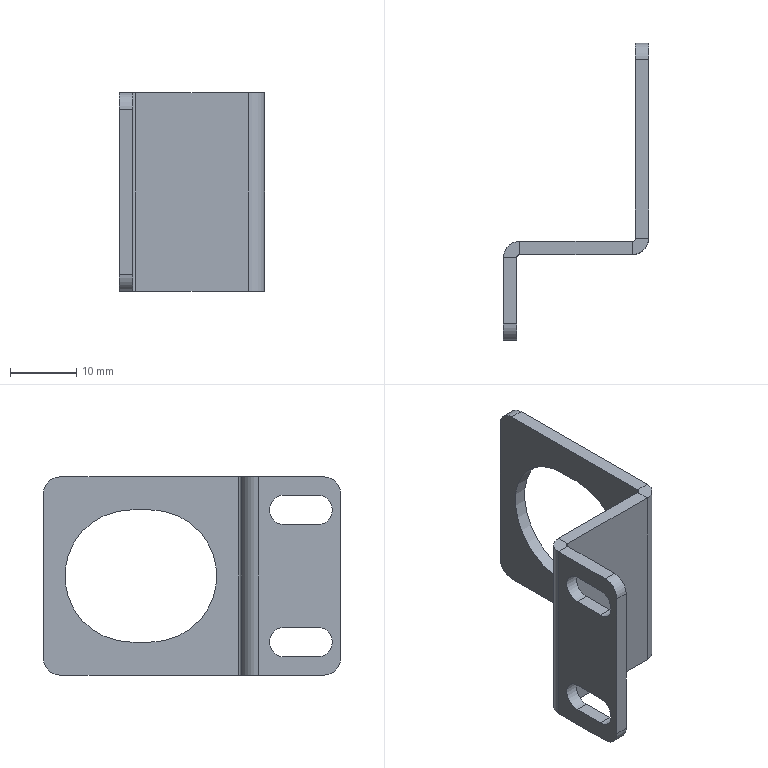Part | STEP file | KF-2212-070-008 | 1 solid | 38 faces | box 22 x 45 x 30 mm | volume 2910 mm3 | plane 24 | cylinder 14 | commonest cylinder face diameters 5 x6 4.5 x4 1 x2 20 x2
STEP:
#1=CARTESIAN_POINT('',(2.5,0.,30.));
#2=VERTEX_POINT('',#1);
#3=CARTESIAN_POINT('',(2.5,-2.,30.));
#4=VERTEX_POINT('',#3);
#5=CARTESIAN_POINT('',(2.5,0.,30.));
#6=DIRECTION('',(0.,-1.,0.));
#7=VECTOR('',#6,1000.);
#8=LINE('',#5,#7);
#9=EDGE_CURVE('',#2,#4,#8,.T.);
#10=ORIENTED_EDGE('',*,*,#9,.F.);
#11=CARTESIAN_POINT('',(0.,-2.5,30.));
#12=VERTEX_POINT('',#11);
#13=CARTESIAN_POINT('',(2.5,-2.5,30.));
#14=DIRECTION('',(0.,0.,-1.));
#15=DIRECTION('',(1.,0.,0.));
#16=AXIS2_PLACEMENT_3D('',#13,#14,#15);
#17=CIRCLE('',#16,2.5);
#18=EDGE_CURVE('',#12,#2,#17,.T.);
#19=ORIENTED_EDGE('',*,*,#18,.F.);
#20=CARTESIAN_POINT('',(2.,-2.5,30.));
#21=VERTEX_POINT('',#20);
#22=CARTESIAN_POINT('',(2.,-2.5,30.));
#23=DIRECTION('',(-1.,0.,0.));
#24=VECTOR('',#23,1000.);
#25=LINE('',#22,#24);
#26=EDGE_CURVE('',#21,#12,#25,.T.);
#27=ORIENTED_EDGE('',*,*,#26,.F.);
#28=CARTESIAN_POINT('',(2.5,-2.5,30.));
#29=DIRECTION('',(0.,0.,-1.));
#30=DIRECTION('',(1.,0.,0.));
#31=AXIS2_PLACEMENT_3D('',#28,#29,#30);
#32=CIRCLE('',#31,0.5);
#33=EDGE_CURVE('',#21,#4,#32,.T.);
#34=ORIENTED_EDGE('',*,*,#33,.T.);
#35=EDGE_LOOP('',(#10,#19,#27,#34));
#36=FACE_OUTER_BOUND('',#35,.T.);
#37=CARTESIAN_POINT('',(2.5,0.,30.));
#38=DIRECTION('',(0.,0.,1.));
#39=DIRECTION('',(1.,0.,0.));
#40=AXIS2_PLACEMENT_3D('',#37,#38,#39);
#41=PLANE('',#40);
#42=ADVANCED_FACE('',(#36),#41,.T.);
#43=CARTESIAN_POINT('',(19.5,0.,30.));
#44=VERTEX_POINT('',#43);
#45=CARTESIAN_POINT('',(0.,0.,30.));
#46=DIRECTION('',(1.,0.,0.));
#47=VECTOR('',#46,1000.);
#48=LINE('',#45,#47);
#49=EDGE_CURVE('',#2,#44,#48,.T.);
#50=ORIENTED_EDGE('',*,*,#49,.F.);
#51=ORIENTED_EDGE('',*,*,#9,.T.);
#52=CARTESIAN_POINT('',(19.5,-2.,30.));
#53=VERTEX_POINT('',#52);
#54=CARTESIAN_POINT('',(0.,-2.,30.));
#55=DIRECTION('',(1.,0.,0.));
#56=VECTOR('',#55,1000.);
#57=LINE('',#54,#56);
#58=EDGE_CURVE('',#4,#53,#57,.T.);
#59=ORIENTED_EDGE('',*,*,#58,.T.);
#60=CARTESIAN_POINT('',(19.5,-2.,30.));
#61=DIRECTION('',(0.,1.,0.));
#62=VECTOR('',#61,1000.);
#63=LINE('',#60,#62);
#64=EDGE_CURVE('',#53,#44,#63,.T.);
#65=ORIENTED_EDGE('',*,*,#64,.T.);
#66=EDGE_LOOP('',(#50,#51,#59,#65));
#67=FACE_OUTER_BOUND('',#66,.T.);
#68=CARTESIAN_POINT('',(2.,-2.5,30.));
#69=DIRECTION('',(0.,0.,1.));
#70=DIRECTION('',(1.,0.,0.));
#71=AXIS2_PLACEMENT_3D('',#68,#69,#70);
#72=PLANE('',#71);
#73=ADVANCED_FACE('',(#67),#72,.T.);
#74=CARTESIAN_POINT('',(0.,-2.5,0.));
#75=VERTEX_POINT('',#74);
#76=CARTESIAN_POINT('',(2.,-2.5,0.));
#77=VERTEX_POINT('',#76);
#78=CARTESIAN_POINT('',(0.,-2.5,0.));
#79=DIRECTION('',(1.,0.,0.));
#80=VECTOR('',#79,1000.);
#81=LINE('',#78,#80);
#82=EDGE_CURVE('',#75,#77,#81,.T.);
#83=ORIENTED_EDGE('',*,*,#82,.F.);
#84=CARTESIAN_POINT('',(2.5,0.,0.));
#85=VERTEX_POINT('',#84);
#86=CARTESIAN_POINT('',(2.5,-2.5,0.));
#87=DIRECTION('',(0.,0.,-1.));
#88=DIRECTION('',(1.,0.,0.));
#89=AXIS2_PLACEMENT_3D('',#86,#87,#88);
#90=CIRCLE('',#89,2.5);
#91=EDGE_CURVE('',#75,#85,#90,.T.);
#92=ORIENTED_EDGE('',*,*,#91,.T.);
#93=CARTESIAN_POINT('',(2.5,-2.,0.));
#94=VERTEX_POINT('',#93);
#95=CARTESIAN_POINT('',(2.5,-2.,0.));
#96=DIRECTION('',(0.,1.,0.));
#97=VECTOR('',#96,1000.);
#98=LINE('',#95,#97);
#99=EDGE_CURVE('',#94,#85,#98,.T.);
#100=ORIENTED_EDGE('',*,*,#99,.F.);
#101=CARTESIAN_POINT('',(2.5,-2.5,0.));
#102=DIRECTION('',(0.,0.,-1.));
#103=DIRECTION('',(1.,0.,0.));
#104=AXIS2_PLACEMENT_3D('',#101,#102,#103);
#105=CIRCLE('',#104,0.5);
#106=EDGE_CURVE('',#77,#94,#105,.T.);
#107=ORIENTED_EDGE('',*,*,#106,.F.);
#108=EDGE_LOOP('',(#83,#92,#100,#107));
#109=FACE_OUTER_BOUND('',#108,.T.);
#110=CARTESIAN_POINT('',(0.,-2.5,0.));
#111=DIRECTION('',(0.,0.,-1.));
#112=DIRECTION('',(-1.,0.,0.));
#113=AXIS2_PLACEMENT_3D('',#110,#111,#112);
#114=PLANE('',#113);
#115=ADVANCED_FACE('',(#109),#114,.T.);
#116=CARTESIAN_POINT('',(2.,-12.5,0.));
#117=VERTEX_POINT('',#116);
#118=CARTESIAN_POINT('',(2.,-15.,0.));
#119=DIRECTION('',(0.,1.,0.));
#120=VECTOR('',#119,1000.);
#121=LINE('',#118,#120);
#122=EDGE_CURVE('',#117,#77,#121,.T.);
#123=ORIENTED_EDGE('',*,*,#122,.F.);
#124=CARTESIAN_POINT('',(0.,-12.5,0.));
#125=VERTEX_POINT('',#124);
#126=CARTESIAN_POINT('',(2.5,-12.5,0.));
#127=DIRECTION('',(-1.,0.,0.));
#128=VECTOR('',#127,1000.);
#129=LINE('',#126,#128);
#130=EDGE_CURVE('',#117,#125,#129,.T.);
#131=ORIENTED_EDGE('',*,*,#130,.T.);
#132=CARTESIAN_POINT('',(0.,-15.,0.));
#133=DIRECTION('',(0.,1.,0.));
#134=VECTOR('',#133,1000.);
#135=LINE('',#132,#134);
#136=EDGE_CURVE('',#125,#75,#135,.T.);
#137=ORIENTED_EDGE('',*,*,#136,.T.);
#138=ORIENTED_EDGE('',*,*,#82,.T.);
#139=EDGE_LOOP('',(#123,#131,#137,#138));
#140=FACE_OUTER_BOUND('',#139,.T.);
#141=CARTESIAN_POINT('',(2.5,-2.,0.));
#142=DIRECTION('',(0.,0.,-1.));
#143=DIRECTION('',(-1.,0.,0.));
#144=AXIS2_PLACEMENT_3D('',#141,#142,#143);
#145=PLANE('',#144);
#146=ADVANCED_FACE('',(#140),#145,.T.);
#147=CARTESIAN_POINT('',(20.,0.5,30.));
#148=VERTEX_POINT('',#147);
#149=CARTESIAN_POINT('',(22.,0.5,30.));
#150=VERTEX_POINT('',#149);
#151=CARTESIAN_POINT('',(20.,0.5,30.));
#152=DIRECTION('',(1.,0.,0.));
#153=VECTOR('',#152,1000.);
#154=LINE('',#151,#153);
#155=EDGE_CURVE('',#148,#150,#154,.T.);
#156=ORIENTED_EDGE('',*,*,#155,.F.);
#157=CARTESIAN_POINT('',(19.5,0.5,30.));
#158=DIRECTION('',(0.,0.,1.));
#159=DIRECTION('',(-1.,0.,0.));
#160=AXIS2_PLACEMENT_3D('',#157,#158,#159);
#161=CIRCLE('',#160,0.5);
#162=EDGE_CURVE('',#44,#148,#161,.T.);
#163=ORIENTED_EDGE('',*,*,#162,.F.);
#164=ORIENTED_EDGE('',*,*,#64,.F.);
#165=CARTESIAN_POINT('',(19.5,0.5,30.));
#166=DIRECTION('',(0.,0.,1.));
#167=DIRECTION('',(1.,0.,0.));
#168=AXIS2_PLACEMENT_3D('',#165,#166,#167);
#169=CIRCLE('',#168,2.5);
#170=EDGE_CURVE('',#53,#150,#169,.T.);
#171=ORIENTED_EDGE('',*,*,#170,.T.);
#172=EDGE_LOOP('',(#156,#163,#164,#171));
#173=FACE_OUTER_BOUND('',#172,.T.);
#174=CARTESIAN_POINT('',(20.,0.5,30.));
#175=DIRECTION('',(0.,0.,1.));
#176=DIRECTION('',(1.,0.,0.));
#177=AXIS2_PLACEMENT_3D('',#174,#175,#176);
#178=PLANE('',#177);
#179=ADVANCED_FACE('',(#173),#178,.T.);
#180=CARTESIAN_POINT('',(22.,27.5,30.));
#181=VERTEX_POINT('',#180);
#182=CARTESIAN_POINT('',(22.,0.,30.));
#183=DIRECTION('',(0.,1.,0.));
#184=VECTOR('',#183,1000.);
#185=LINE('',#182,#184);
#186=EDGE_CURVE('',#150,#181,#185,.T.);
#187=ORIENTED_EDGE('',*,*,#186,.T.);
#188=CARTESIAN_POINT('',(20.,27.5,30.));
#189=VERTEX_POINT('',#188);
#190=CARTESIAN_POINT('',(19.5,27.5,30.));
#191=DIRECTION('',(-1.,0.,0.));
#192=VECTOR('',#191,1000.);
#193=LINE('',#190,#192);
#194=EDGE_CURVE('',#181,#189,#193,.T.);
#195=ORIENTED_EDGE('',*,*,#194,.T.);
#196=CARTESIAN_POINT('',(20.,0.,30.));
#197=DIRECTION('',(0.,1.,0.));
#198=VECTOR('',#197,1000.);
#199=LINE('',#196,#198);
#200=EDGE_CURVE('',#148,#189,#199,.T.);
#201=ORIENTED_EDGE('',*,*,#200,.F.);
#202=ORIENTED_EDGE('',*,*,#155,.T.);
#203=EDGE_LOOP('',(#187,#195,#201,#202));
#204=FACE_OUTER_BOUND('',#203,.T.);
#205=CARTESIAN_POINT('',(19.5,-2.,30.));
#206=DIRECTION('',(0.,0.,1.));
#207=DIRECTION('',(1.,0.,0.));
#208=AXIS2_PLACEMENT_3D('',#205,#206,#207);
#209=PLANE('',#208);
#210=ADVANCED_FACE('',(#204),#209,.T.);
#211=CARTESIAN_POINT('',(19.5,0.,0.));
#212=VERTEX_POINT('',#211);
#213=CARTESIAN_POINT('',(19.5,-2.,0.));
#214=VERTEX_POINT('',#213);
#215=CARTESIAN_POINT('',(19.5,0.,0.));
#216=DIRECTION('',(0.,-1.,0.));
#217=VECTOR('',#216,1000.);
#218=LINE('',#215,#217);
#219=EDGE_CURVE('',#212,#214,#218,.T.);
#220=ORIENTED_EDGE('',*,*,#219,.F.);
#221=CARTESIAN_POINT('',(20.,0.5,0.));
#222=VERTEX_POINT('',#221);
#223=CARTESIAN_POINT('',(19.5,0.5,0.));
#224=DIRECTION('',(0.,0.,1.));
#225=DIRECTION('',(-1.,0.,0.));
#226=AXIS2_PLACEMENT_3D('',#223,#224,#225);
#227=CIRCLE('',#226,0.5);
#228=EDGE_CURVE('',#212,#222,#227,.T.);
#229=ORIENTED_EDGE('',*,*,#228,.T.);
#230=CARTESIAN_POINT('',(22.,0.5,0.));
#231=VERTEX_POINT('',#230);
#232=CARTESIAN_POINT('',(22.,0.5,0.));
#233=DIRECTION('',(-1.,0.,0.));
#234=VECTOR('',#233,1000.);
#235=LINE('',#232,#234);
#236=EDGE_CURVE('',#231,#222,#235,.T.);
#237=ORIENTED_EDGE('',*,*,#236,.F.);
#238=CARTESIAN_POINT('',(19.5,0.5,0.));
#239=DIRECTION('',(0.,0.,1.));
#240=DIRECTION('',(1.,0.,0.));
#241=AXIS2_PLACEMENT_3D('',#238,#239,#240);
#242=CIRCLE('',#241,2.5);
#243=EDGE_CURVE('',#214,#231,#242,.T.);
#244=ORIENTED_EDGE('',*,*,#243,.F.);
#245=EDGE_LOOP('',(#220,#229,#237,#244));
#246=FACE_OUTER_BOUND('',#245,.T.);
#247=CARTESIAN_POINT('',(19.5,0.,0.));
#248=DIRECTION('',(0.,0.,-1.));
#249=DIRECTION('',(-1.,0.,0.));
#250=AXIS2_PLACEMENT_3D('',#247,#248,#249);
#251=PLANE('',#250);
#252=ADVANCED_FACE('',(#246),#251,.T.);
#253=CARTESIAN_POINT('',(0.,0.,0.));
#254=DIRECTION('',(1.,0.,0.));
#255=VECTOR('',#254,1000.);
#256=LINE('',#253,#255);
#257=EDGE_CURVE('',#85,#212,#256,.T.);
#258=ORIENTED_EDGE('',*,*,#257,.T.);
#259=ORIENTED_EDGE('',*,*,#219,.T.);
#260=CARTESIAN_POINT('',(0.,-2.,0.));
#261=DIRECTION('',(1.,0.,0.));
#262=VECTOR('',#261,1000.);
#263=LINE('',#260,#262);
#264=EDGE_CURVE('',#94,#214,#263,.T.);
#265=ORIENTED_EDGE('',*,*,#264,.F.);
#266=ORIENTED_EDGE('',*,*,#99,.T.);
#267=EDGE_LOOP('',(#258,#259,#265,#266));
#268=FACE_OUTER_BOUND('',#267,.T.);
#269=CARTESIAN_POINT('',(22.,0.5,0.));
#270=DIRECTION('',(0.,0.,-1.));
#271=DIRECTION('',(-1.,0.,0.));
#272=AXIS2_PLACEMENT_3D('',#269,#270,#271);
#273=PLANE('',#272);
#274=ADVANCED_FACE('',(#268),#273,.T.);
#275=CARTESIAN_POINT('',(22.,16.75,25.));
#276=VERTEX_POINT('',#275);
#277=CARTESIAN_POINT('',(22.,13.75,25.));
#278=VERTEX_POINT('',#277);
#279=CARTESIAN_POINT('',(22.,16.75,25.));
#280=DIRECTION('',(0.,-1.,0.));
#281=VECTOR('',#280,1000.);
#282=LINE('',#279,#281);
#283=EDGE_CURVE('',#276,#278,#282,.T.);
#284=ORIENTED_EDGE('',*,*,#283,.F.);
#285=CARTESIAN_POINT('',(22.,16.75,5.));
#286=VERTEX_POINT('',#285);
#287=CARTESIAN_POINT('',(22.,16.75,15.));
#288=DIRECTION('',(1.,0.,0.));
#289=DIRECTION('',(0.,0.,-1.));
#290=AXIS2_PLACEMENT_3D('',#287,#288,#289);
#291=CIRCLE('',#290,10.);
#292=EDGE_CURVE('',#286,#276,#291,.T.);
#293=ORIENTED_EDGE('',*,*,#292,.F.);
#294=CARTESIAN_POINT('',(22.,13.75,5.));
#295=VERTEX_POINT('',#294);
#296=CARTESIAN_POINT('',(22.,16.75,5.));
#297=DIRECTION('',(0.,1.,0.));
#298=VECTOR('',#297,1000.);
#299=LINE('',#296,#298);
#300=EDGE_CURVE('',#295,#286,#299,.T.);
#301=ORIENTED_EDGE('',*,*,#300,.F.);
#302=CARTESIAN_POINT('',(22.,13.75,15.));
#303=DIRECTION('',(1.,0.,0.));
#304=DIRECTION('',(0.,0.,-1.));
#305=AXIS2_PLACEMENT_3D('',#302,#303,#304);
#306=CIRCLE('',#305,10.);
#307=EDGE_CURVE('',#278,#295,#306,.T.);
#308=ORIENTED_EDGE('',*,*,#307,.F.);
#309=EDGE_LOOP('',(#284,#293,#301,#308));
#310=FACE_BOUND('',#309,.T.);
#311=CARTESIAN_POINT('',(22.,27.5,0.));
#312=VERTEX_POINT('',#311);
#313=CARTESIAN_POINT('',(22.,0.,0.));
#314=DIRECTION('',(0.,1.,0.));
#315=VECTOR('',#314,1000.);
#316=LINE('',#313,#315);
#317=EDGE_CURVE('',#231,#312,#316,.T.);
#318=ORIENTED_EDGE('',*,*,#317,.T.);
#319=CARTESIAN_POINT('',(22.,30.,2.5));
#320=VERTEX_POINT('',#319);
#321=CARTESIAN_POINT('',(22.,27.5,2.5));
#322=DIRECTION('',(1.,0.,0.));
#323=DIRECTION('',(0.,0.,1.));
#324=AXIS2_PLACEMENT_3D('',#321,#322,#323);
#325=CIRCLE('',#324,2.5);
#326=EDGE_CURVE('',#312,#320,#325,.T.);
#327=ORIENTED_EDGE('',*,*,#326,.T.);
#328=CARTESIAN_POINT('',(22.,30.,27.5));
#329=VERTEX_POINT('',#328);
#330=CARTESIAN_POINT('',(22.,30.,30.));
#331=DIRECTION('',(0.,0.,-1.));
#332=VECTOR('',#331,1000.);
#333=LINE('',#330,#332);
#334=EDGE_CURVE('',#329,#320,#333,.T.);
#335=ORIENTED_EDGE('',*,*,#334,.F.);
#336=CARTESIAN_POINT('',(22.,27.5,27.5));
#337=DIRECTION('',(1.,0.,0.));
#338=DIRECTION('',(0.,0.,1.));
#339=AXIS2_PLACEMENT_3D('',#336,#337,#338);
#340=CIRCLE('',#339,2.5);
#341=EDGE_CURVE('',#329,#181,#340,.T.);
#342=ORIENTED_EDGE('',*,*,#341,.T.);
#343=ORIENTED_EDGE('',*,*,#186,.F.);
#344=CARTESIAN_POINT('',(22.,0.5,30.));
#345=DIRECTION('',(0.,0.,-1.));
#346=VECTOR('',#345,1000.);
#347=LINE('',#344,#346);
#348=EDGE_CURVE('',#150,#231,#347,.T.);
#349=ORIENTED_EDGE('',*,*,#348,.T.);
#350=EDGE_LOOP('',(#318,#327,#335,#342,#343,#349));
#351=FACE_OUTER_BOUND('',#350,.T.);
#352=CARTESIAN_POINT('',(22.,0.,30.));
#353=DIRECTION('',(-1.,0.,0.));
#354=DIRECTION('',(0.,0.,1.));
#355=AXIS2_PLACEMENT_3D('',#352,#353,#354);
#356=PLANE('',#355);
#357=ADVANCED_FACE('',(#310,#351),#356,.F.);
#358=ORIENTED_EDGE('',*,*,#334,.T.);
#359=CARTESIAN_POINT('',(20.,30.,2.5));
#360=VERTEX_POINT('',#359);
#361=CARTESIAN_POINT('',(20.,30.,2.5));
#362=DIRECTION('',(-1.,0.,0.));
#363=VECTOR('',#362,1000.);
#364=LINE('',#361,#363);
#365=EDGE_CURVE('',#320,#360,#364,.T.);
#366=ORIENTED_EDGE('',*,*,#365,.T.);
#367=CARTESIAN_POINT('',(20.,30.,27.5));
#368=VERTEX_POINT('',#367);
#369=CARTESIAN_POINT('',(20.,30.,30.));
#370=DIRECTION('',(0.,0.,-1.));
#371=VECTOR('',#370,1000.);
#372=LINE('',#369,#371);
#373=EDGE_CURVE('',#368,#360,#372,.T.);
#374=ORIENTED_EDGE('',*,*,#373,.F.);
#375=CARTESIAN_POINT('',(20.,30.,27.5));
#376=DIRECTION('',(1.,0.,0.));
#377=VECTOR('',#376,1000.);
#378=LINE('',#375,#377);
#379=EDGE_CURVE('',#368,#329,#378,.T.);
#380=ORIENTED_EDGE('',*,*,#379,.T.);
#381=EDGE_LOOP('',(#358,#366,#374,#380));
#382=FACE_OUTER_BOUND('',#381,.T.);
#383=CARTESIAN_POINT('',(20.,30.,30.));
#384=DIRECTION('',(0.,1.,0.));
#385=DIRECTION('',(0.,0.,1.));
#386=AXIS2_PLACEMENT_3D('',#383,#384,#385);
#387=PLANE('',#386);
#388=ADVANCED_FACE('',(#382),#387,.T.);
#389=CARTESIAN_POINT('',(20.,16.75,25.));
#390=VERTEX_POINT('',#389);
#391=CARTESIAN_POINT('',(20.,16.75,5.));
#392=VERTEX_POINT('',#391);
#393=CARTESIAN_POINT('',(20.,16.75,15.));
#394=DIRECTION('',(-1.,0.,0.));
#395=DIRECTION('',(0.,0.,1.));
#396=AXIS2_PLACEMENT_3D('',#393,#394,#395);
#397=CIRCLE('',#396,10.);
#398=EDGE_CURVE('',#390,#392,#397,.T.);
#399=ORIENTED_EDGE('',*,*,#398,.F.);
#400=CARTESIAN_POINT('',(20.,13.75,25.));
#401=VERTEX_POINT('',#400);
#402=CARTESIAN_POINT('',(20.,0.,25.));
#403=DIRECTION('',(0.,1.,0.));
#404=VECTOR('',#403,1000.);
#405=LINE('',#402,#404);
#406=EDGE_CURVE('',#401,#390,#405,.T.);
#407=ORIENTED_EDGE('',*,*,#406,.F.);
#408=CARTESIAN_POINT('',(20.,13.75,5.));
#409=VERTEX_POINT('',#408);
#410=CARTESIAN_POINT('',(20.,13.75,15.));
#411=DIRECTION('',(-1.,0.,0.));
#412=DIRECTION('',(0.,0.,1.));
#413=AXIS2_PLACEMENT_3D('',#410,#411,#412);
#414=CIRCLE('',#413,10.);
#415=EDGE_CURVE('',#409,#401,#414,.T.);
#416=ORIENTED_EDGE('',*,*,#415,.F.);
#417=CARTESIAN_POINT('',(20.,0.,5.));
#418=DIRECTION('',(0.,-1.,0.));
#419=VECTOR('',#418,1000.);
#420=LINE('',#417,#419);
#421=EDGE_CURVE('',#392,#409,#420,.T.);
#422=ORIENTED_EDGE('',*,*,#421,.F.);
#423=EDGE_LOOP('',(#399,#407,#416,#422));
#424=FACE_BOUND('',#423,.T.);
#425=ORIENTED_EDGE('',*,*,#373,.T.);
#426=CARTESIAN_POINT('',(20.,27.5,0.));
#427=VERTEX_POINT('',#426);
#428=CARTESIAN_POINT('',(20.,27.5,2.5));
#429=DIRECTION('',(-1.,0.,0.));
#430=DIRECTION('',(0.,0.,1.));
#431=AXIS2_PLACEMENT_3D('',#428,#429,#430);
#432=CIRCLE('',#431,2.5);
#433=EDGE_CURVE('',#360,#427,#432,.T.);
#434=ORIENTED_EDGE('',*,*,#433,.T.);
#435=CARTESIAN_POINT('',(20.,0.,0.));
#436=DIRECTION('',(0.,1.,0.));
#437=VECTOR('',#436,1000.);
#438=LINE('',#435,#437);
#439=EDGE_CURVE('',#222,#427,#438,.T.);
#440=ORIENTED_EDGE('',*,*,#439,.F.);
#441=CARTESIAN_POINT('',(20.,0.5,30.));
#442=DIRECTION('',(0.,0.,-1.));
#443=VECTOR('',#442,1000.);
#444=LINE('',#441,#443);
#445=EDGE_CURVE('',#148,#222,#444,.T.);
#446=ORIENTED_EDGE('',*,*,#445,.F.);
#447=ORIENTED_EDGE('',*,*,#200,.T.);
#448=CARTESIAN_POINT('',(20.,27.5,27.5));
#449=DIRECTION('',(-1.,0.,0.));
#450=DIRECTION('',(0.,0.,1.));
#451=AXIS2_PLACEMENT_3D('',#448,#449,#450);
#452=CIRCLE('',#451,2.5);
#453=EDGE_CURVE('',#189,#368,#452,.T.);
#454=ORIENTED_EDGE('',*,*,#453,.T.);
#455=EDGE_LOOP('',(#425,#434,#440,#446,#447,#454));
#456=FACE_OUTER_BOUND('',#455,.T.);
#457=CARTESIAN_POINT('',(20.,0.,30.));
#458=DIRECTION('',(-1.,0.,0.));
#459=DIRECTION('',(0.,0.,1.));
#460=AXIS2_PLACEMENT_3D('',#457,#458,#459);
#461=PLANE('',#460);
#462=ADVANCED_FACE('',(#424,#456),#461,.T.);
#463=ORIENTED_EDGE('',*,*,#228,.F.);
#464=CARTESIAN_POINT('',(19.5,0.,30.));
#465=DIRECTION('',(0.,0.,-1.));
#466=VECTOR('',#465,1000.);
#467=LINE('',#464,#466);
#468=EDGE_CURVE('',#44,#212,#467,.T.);
#469=ORIENTED_EDGE('',*,*,#468,.F.);
#470=ORIENTED_EDGE('',*,*,#162,.T.);
#471=ORIENTED_EDGE('',*,*,#445,.T.);
#472=EDGE_LOOP('',(#463,#469,#470,#471));
#473=FACE_OUTER_BOUND('',#472,.T.);
#474=CARTESIAN_POINT('',(19.5,0.5,30.));
#475=DIRECTION('',(0.,0.,-1.));
#476=DIRECTION('',(-1.,0.,0.));
#477=AXIS2_PLACEMENT_3D('',#474,#475,#476);
#478=CYLINDRICAL_SURFACE('',#477,0.5);
#479=ADVANCED_FACE('',(#473),#478,.F.);
#480=ORIENTED_EDGE('',*,*,#257,.F.);
#481=CARTESIAN_POINT('',(2.5,0.,30.));
#482=DIRECTION('',(0.,0.,-1.));
#483=VECTOR('',#482,1000.);
#484=LINE('',#481,#483);
#485=EDGE_CURVE('',#2,#85,#484,.T.);
#486=ORIENTED_EDGE('',*,*,#485,.F.);
#487=ORIENTED_EDGE('',*,*,#49,.T.);
#488=ORIENTED_EDGE('',*,*,#468,.T.);
#489=EDGE_LOOP('',(#480,#486,#487,#488));
#490=FACE_OUTER_BOUND('',#489,.T.);
#491=CARTESIAN_POINT('',(0.,0.,30.));
#492=DIRECTION('',(0.,1.,0.));
#493=DIRECTION('',(0.,0.,1.));
#494=AXIS2_PLACEMENT_3D('',#491,#492,#493);
#495=PLANE('',#494);
#496=ADVANCED_FACE('',(#490),#495,.T.);
#497=ORIENTED_EDGE('',*,*,#91,.F.);
#498=CARTESIAN_POINT('',(0.,-2.5,30.));
#499=DIRECTION('',(0.,0.,-1.));
#500=VECTOR('',#499,1000.);
#501=LINE('',#498,#500);
#502=EDGE_CURVE('',#12,#75,#501,.T.);
#503=ORIENTED_EDGE('',*,*,#502,.F.);
#504=ORIENTED_EDGE('',*,*,#18,.T.);
#505=ORIENTED_EDGE('',*,*,#485,.T.);
#506=EDGE_LOOP('',(#497,#503,#504,#505));
#507=FACE_OUTER_BOUND('',#506,.T.);
#508=CARTESIAN_POINT('',(2.5,-2.5,30.));
#509=DIRECTION('',(0.,0.,-1.));
#510=DIRECTION('',(-1.,0.,0.));
#511=AXIS2_PLACEMENT_3D('',#508,#509,#510);
#512=CYLINDRICAL_SURFACE('',#511,2.5);
#513=ADVANCED_FACE('',(#507),#512,.T.);
#514=CARTESIAN_POINT('',(0.,-6.5,7.25));
#515=VERTEX_POINT('',#514);
#516=CARTESIAN_POINT('',(0.,-6.5,2.75));
#517=VERTEX_POINT('',#516);
#518=CARTESIAN_POINT('',(0.,-6.5,5.));
#519=DIRECTION('',(-1.,0.,0.));
#520=DIRECTION('',(0.,0.,1.));
#521=AXIS2_PLACEMENT_3D('',#518,#519,#520);
#522=CIRCLE('',#521,2.25);
#523=EDGE_CURVE('',#515,#517,#522,.T.);
#524=ORIENTED_EDGE('',*,*,#523,.F.);
#525=CARTESIAN_POINT('',(0.,-11.5,7.25));
#526=VERTEX_POINT('',#525);
#527=CARTESIAN_POINT('',(0.,-6.5,7.25));
#528=DIRECTION('',(0.,1.,0.));
#529=VECTOR('',#528,1000.);
#530=LINE('',#527,#529);
#531=EDGE_CURVE('',#526,#515,#530,.T.);
#532=ORIENTED_EDGE('',*,*,#531,.F.);
#533=CARTESIAN_POINT('',(0.,-11.5,2.75));
#534=VERTEX_POINT('',#533);
#535=CARTESIAN_POINT('',(0.,-11.5,5.));
#536=DIRECTION('',(-1.,0.,0.));
#537=DIRECTION('',(0.,0.,1.));
#538=AXIS2_PLACEMENT_3D('',#535,#536,#537);
#539=CIRCLE('',#538,2.25);
#540=EDGE_CURVE('',#534,#526,#539,.T.);
#541=ORIENTED_EDGE('',*,*,#540,.F.);
#542=CARTESIAN_POINT('',(0.,-6.5,2.75));
#543=DIRECTION('',(0.,-1.,0.));
#544=VECTOR('',#543,1000.);
#545=LINE('',#542,#544);
#546=EDGE_CURVE('',#517,#534,#545,.T.);
#547=ORIENTED_EDGE('',*,*,#546,.F.);
#548=EDGE_LOOP('',(#524,#532,#541,#547));
#549=FACE_BOUND('',#548,.T.);
#550=CARTESIAN_POINT('',(0.,-6.5,27.25));
#551=VERTEX_POINT('',#550);
#552=CARTESIAN_POINT('',(0.,-6.5,22.75));
#553=VERTEX_POINT('',#552);
#554=CARTESIAN_POINT('',(0.,-6.5,25.));
#555=DIRECTION('',(-1.,0.,0.));
#556=DIRECTION('',(0.,0.,1.));
#557=AXIS2_PLACEMENT_3D('',#554,#555,#556);
#558=CIRCLE('',#557,2.25);
#559=EDGE_CURVE('',#551,#553,#558,.T.);
#560=ORIENTED_EDGE('',*,*,#559,.F.);
#561=CARTESIAN_POINT('',(0.,-11.5,27.25));
#562=VERTEX_POINT('',#561);
#563=CARTESIAN_POINT('',(0.,-6.5,27.25));
#564=DIRECTION('',(0.,1.,0.));
#565=VECTOR('',#564,1000.);
#566=LINE('',#563,#565);
#567=EDGE_CURVE('',#562,#551,#566,.T.);
#568=ORIENTED_EDGE('',*,*,#567,.F.);
#569=CARTESIAN_POINT('',(0.,-11.5,22.75));
#570=VERTEX_POINT('',#569);
#571=CARTESIAN_POINT('',(0.,-11.5,25.));
#572=DIRECTION('',(-1.,0.,0.));
#573=DIRECTION('',(0.,0.,1.));
#574=AXIS2_PLACEMENT_3D('',#571,#572,#573);
#575=CIRCLE('',#574,2.25);
#576=EDGE_CURVE('',#570,#562,#575,.T.);
#577=ORIENTED_EDGE('',*,*,#576,.F.);
#578=CARTESIAN_POINT('',(0.,-6.5,22.75));
#579=DIRECTION('',(0.,-1.,0.));
#580=VECTOR('',#579,1000.);
#581=LINE('',#578,#580);
#582=EDGE_CURVE('',#553,#570,#581,.T.);
#583=ORIENTED_EDGE('',*,*,#582,.F.);
#584=EDGE_LOOP('',(#560,#568,#577,#583));
#585=FACE_BOUND('',#584,.T.);
#586=ORIENTED_EDGE('',*,*,#136,.F.);
#587=CARTESIAN_POINT('',(0.,-15.,2.5));
#588=VERTEX_POINT('',#587);
#589=CARTESIAN_POINT('',(0.,-12.5,2.5));
#590=DIRECTION('',(-1.,0.,0.));
#591=DIRECTION('',(0.,0.,1.));
#592=AXIS2_PLACEMENT_3D('',#589,#590,#591);
#593=CIRCLE('',#592,2.5);
#594=EDGE_CURVE('',#125,#588,#593,.T.);
#595=ORIENTED_EDGE('',*,*,#594,.T.);
#596=CARTESIAN_POINT('',(0.,-15.,27.5));
#597=VERTEX_POINT('',#596);
#598=CARTESIAN_POINT('',(0.,-15.,30.));
#599=DIRECTION('',(0.,0.,-1.));
#600=VECTOR('',#599,1000.);
#601=LINE('',#598,#600);
#602=EDGE_CURVE('',#597,#588,#601,.T.);
#603=ORIENTED_EDGE('',*,*,#602,.F.);
#604=CARTESIAN_POINT('',(0.,-12.5,30.));
#605=VERTEX_POINT('',#604);
#606=CARTESIAN_POINT('',(0.,-12.5,27.5));
#607=DIRECTION('',(-1.,0.,0.));
#608=DIRECTION('',(0.,0.,1.));
#609=AXIS2_PLACEMENT_3D('',#606,#607,#608);
#610=CIRCLE('',#609,2.5);
#611=EDGE_CURVE('',#597,#605,#610,.T.);
#612=ORIENTED_EDGE('',*,*,#611,.T.);
#613=CARTESIAN_POINT('',(0.,-15.,30.));
#614=DIRECTION('',(0.,1.,0.));
#615=VECTOR('',#614,1000.);
#616=LINE('',#613,#615);
#617=EDGE_CURVE('',#605,#12,#616,.T.);
#618=ORIENTED_EDGE('',*,*,#617,.T.);
#619=ORIENTED_EDGE('',*,*,#502,.T.);
#620=EDGE_LOOP('',(#586,#595,#603,#612,#618,#619));
#621=FACE_OUTER_BOUND('',#620,.T.);
#622=CARTESIAN_POINT('',(0.,-15.,30.));
#623=DIRECTION('',(-1.,0.,0.));
#624=DIRECTION('',(0.,0.,1.));
#625=AXIS2_PLACEMENT_3D('',#622,#623,#624);
#626=PLANE('',#625);
#627=ADVANCED_FACE('',(#549,#585,#621),#626,.T.);
#628=ORIENTED_EDGE('',*,*,#602,.T.);
#629=CARTESIAN_POINT('',(2.,-15.,2.5));
#630=VERTEX_POINT('',#629);
#631=CARTESIAN_POINT('',(2.,-15.,2.5));
#632=DIRECTION('',(1.,0.,0.));
#633=VECTOR('',#632,1000.);
#634=LINE('',#631,#633);
#635=EDGE_CURVE('',#588,#630,#634,.T.);
#636=ORIENTED_EDGE('',*,*,#635,.T.);
#637=CARTESIAN_POINT('',(2.,-15.,27.5));
#638=VERTEX_POINT('',#637);
#639=CARTESIAN_POINT('',(2.,-15.,30.));
#640=DIRECTION('',(0.,0.,-1.));
#641=VECTOR('',#640,1000.);
#642=LINE('',#639,#641);
#643=EDGE_CURVE('',#638,#630,#642,.T.);
#644=ORIENTED_EDGE('',*,*,#643,.F.);
#645=CARTESIAN_POINT('',(0.,-15.,27.5));
#646=DIRECTION('',(-1.,0.,0.));
#647=VECTOR('',#646,1000.);
#648=LINE('',#645,#647);
#649=EDGE_CURVE('',#638,#597,#648,.T.);
#650=ORIENTED_EDGE('',*,*,#649,.T.);
#651=EDGE_LOOP('',(#628,#636,#644,#650));
#652=FACE_OUTER_BOUND('',#651,.T.);
#653=CARTESIAN_POINT('',(2.,-15.,30.));
#654=DIRECTION('',(0.,-1.,0.));
#655=DIRECTION('',(0.,0.,-1.));
#656=AXIS2_PLACEMENT_3D('',#653,#654,#655);
#657=PLANE('',#656);
#658=ADVANCED_FACE('',(#652),#657,.T.);
#659=CARTESIAN_POINT('',(2.,-11.5,7.25));
#660=VERTEX_POINT('',#659);
#661=CARTESIAN_POINT('',(2.,-6.5,7.25));
#662=VERTEX_POINT('',#661);
#663=CARTESIAN_POINT('',(2.,-15.,7.25));
#664=DIRECTION('',(0.,1.,0.));
#665=VECTOR('',#664,1000.);
#666=LINE('',#663,#665);
#667=EDGE_CURVE('',#660,#662,#666,.T.);
#668=ORIENTED_EDGE('',*,*,#667,.T.);
#669=CARTESIAN_POINT('',(2.,-6.5,2.75));
#670=VERTEX_POINT('',#669);
#671=CARTESIAN_POINT('',(2.,-6.5,5.));
#672=DIRECTION('',(-1.,0.,0.));
#673=DIRECTION('',(0.,0.,1.));
#674=AXIS2_PLACEMENT_3D('',#671,#672,#673);
#675=CIRCLE('',#674,2.25);
#676=EDGE_CURVE('',#662,#670,#675,.T.);
#677=ORIENTED_EDGE('',*,*,#676,.T.);
#678=CARTESIAN_POINT('',(2.,-11.5,2.75));
#679=VERTEX_POINT('',#678);
#680=CARTESIAN_POINT('',(2.,-15.,2.75));
#681=DIRECTION('',(0.,-1.,0.));
#682=VECTOR('',#681,1000.);
#683=LINE('',#680,#682);
#684=EDGE_CURVE('',#670,#679,#683,.T.);
#685=ORIENTED_EDGE('',*,*,#684,.T.);
#686=CARTESIAN_POINT('',(2.,-11.5,5.));
#687=DIRECTION('',(-1.,0.,0.));
#688=DIRECTION('',(0.,0.,1.));
#689=AXIS2_PLACEMENT_3D('',#686,#687,#688);
#690=CIRCLE('',#689,2.25);
#691=EDGE_CURVE('',#679,#660,#690,.T.);
#692=ORIENTED_EDGE('',*,*,#691,.T.);
#693=EDGE_LOOP('',(#668,#677,#685,#692));
#694=FACE_BOUND('',#693,.T.);
#695=CARTESIAN_POINT('',(2.,-11.5,27.25));
#696=VERTEX_POINT('',#695);
#697=CARTESIAN_POINT('',(2.,-6.5,27.25));
#698=VERTEX_POINT('',#697);
#699=CARTESIAN_POINT('',(2.,-15.,27.25));
#700=DIRECTION('',(0.,1.,0.));
#701=VECTOR('',#700,1000.);
#702=LINE('',#699,#701);
#703=EDGE_CURVE('',#696,#698,#702,.T.);
#704=ORIENTED_EDGE('',*,*,#703,.T.);
#705=CARTESIAN_POINT('',(2.,-6.5,22.75));
#706=VERTEX_POINT('',#705);
#707=CARTESIAN_POINT('',(2.,-6.5,25.));
#708=DIRECTION('',(-1.,0.,0.));
#709=DIRECTION('',(0.,0.,1.));
#710=AXIS2_PLACEMENT_3D('',#707,#708,#709);
#711=CIRCLE('',#710,2.25);
#712=EDGE_CURVE('',#698,#706,#711,.T.);
#713=ORIENTED_EDGE('',*,*,#712,.T.);
#714=CARTESIAN_POINT('',(2.,-11.5,22.75));
#715=VERTEX_POINT('',#714);
#716=CARTESIAN_POINT('',(2.,-15.,22.75));
#717=DIRECTION('',(0.,-1.,0.));
#718=VECTOR('',#717,1000.);
#719=LINE('',#716,#718);
#720=EDGE_CURVE('',#706,#715,#719,.T.);
#721=ORIENTED_EDGE('',*,*,#720,.T.);
#722=CARTESIAN_POINT('',(2.,-11.5,25.));
#723=DIRECTION('',(-1.,0.,0.));
#724=DIRECTION('',(0.,0.,1.));
#725=AXIS2_PLACEMENT_3D('',#722,#723,#724);
#726=CIRCLE('',#725,2.25);
#727=EDGE_CURVE('',#715,#696,#726,.T.);
#728=ORIENTED_EDGE('',*,*,#727,.T.);
#729=EDGE_LOOP('',(#704,#713,#721,#728));
#730=FACE_BOUND('',#729,.T.);
#731=ORIENTED_EDGE('',*,*,#643,.T.);
#732=CARTESIAN_POINT('',(2.,-12.5,2.5));
#733=DIRECTION('',(1.,0.,0.));
#734=DIRECTION('',(0.,0.,1.));
#735=AXIS2_PLACEMENT_3D('',#732,#733,#734);
#736=CIRCLE('',#735,2.5);
#737=EDGE_CURVE('',#630,#117,#736,.T.);
#738=ORIENTED_EDGE('',*,*,#737,.T.);
#739=ORIENTED_EDGE('',*,*,#122,.T.);
#740=CARTESIAN_POINT('',(2.,-2.5,30.));
#741=DIRECTION('',(0.,0.,-1.));
#742=VECTOR('',#741,1000.);
#743=LINE('',#740,#742);
#744=EDGE_CURVE('',#21,#77,#743,.T.);
#745=ORIENTED_EDGE('',*,*,#744,.F.);
#746=CARTESIAN_POINT('',(2.,-12.5,30.));
#747=VERTEX_POINT('',#746);
#748=CARTESIAN_POINT('',(2.,-15.,30.));
#749=DIRECTION('',(0.,1.,0.));
#750=VECTOR('',#749,1000.);
#751=LINE('',#748,#750);
#752=EDGE_CURVE('',#747,#21,#751,.T.);
#753=ORIENTED_EDGE('',*,*,#752,.F.);
#754=CARTESIAN_POINT('',(2.,-12.5,27.5));
#755=DIRECTION('',(1.,0.,0.));
#756=DIRECTION('',(0.,0.,1.));
#757=AXIS2_PLACEMENT_3D('',#754,#755,#756);
#758=CIRCLE('',#757,2.5);
#759=EDGE_CURVE('',#747,#638,#758,.T.);
#760=ORIENTED_EDGE('',*,*,#759,.T.);
#761=EDGE_LOOP('',(#731,#738,#739,#745,#753,#760));
#762=FACE_OUTER_BOUND('',#761,.T.);
#763=CARTESIAN_POINT('',(2.,-15.,30.));
#764=DIRECTION('',(-1.,0.,0.));
#765=DIRECTION('',(0.,0.,1.));
#766=AXIS2_PLACEMENT_3D('',#763,#764,#765);
#767=PLANE('',#766);
#768=ADVANCED_FACE('',(#694,#730,#762),#767,.F.);
#769=ORIENTED_EDGE('',*,*,#106,.T.);
#770=CARTESIAN_POINT('',(2.5,-2.,30.));
#771=DIRECTION('',(0.,0.,-1.));
#772=VECTOR('',#771,1000.);
#773=LINE('',#770,#772);
#774=EDGE_CURVE('',#4,#94,#773,.T.);
#775=ORIENTED_EDGE('',*,*,#774,.F.);
#776=ORIENTED_EDGE('',*,*,#33,.F.);
#777=ORIENTED_EDGE('',*,*,#744,.T.);
#778=EDGE_LOOP('',(#769,#775,#776,#777));
#779=FACE_OUTER_BOUND('',#778,.T.);
#780=CARTESIAN_POINT('',(2.5,-2.5,30.));
#781=DIRECTION('',(0.,0.,-1.));
#782=DIRECTION('',(-1.,0.,0.));
#783=AXIS2_PLACEMENT_3D('',#780,#781,#782);
#784=CYLINDRICAL_SURFACE('',#783,0.5);
#785=ADVANCED_FACE('',(#779),#784,.F.);
#786=ORIENTED_EDGE('',*,*,#264,.T.);
#787=CARTESIAN_POINT('',(19.5,-2.,30.));
#788=DIRECTION('',(0.,0.,-1.));
#789=VECTOR('',#788,1000.);
#790=LINE('',#787,#789);
#791=EDGE_CURVE('',#53,#214,#790,.T.);
#792=ORIENTED_EDGE('',*,*,#791,.F.);
#793=ORIENTED_EDGE('',*,*,#58,.F.);
#794=ORIENTED_EDGE('',*,*,#774,.T.);
#795=EDGE_LOOP('',(#786,#792,#793,#794));
#796=FACE_OUTER_BOUND('',#795,.T.);
#797=CARTESIAN_POINT('',(0.,-2.,30.));
#798=DIRECTION('',(0.,1.,0.));
#799=DIRECTION('',(0.,0.,1.));
#800=AXIS2_PLACEMENT_3D('',#797,#798,#799);
#801=PLANE('',#800);
#802=ADVANCED_FACE('',(#796),#801,.F.);
#803=ORIENTED_EDGE('',*,*,#243,.T.);
#804=ORIENTED_EDGE('',*,*,#348,.F.);
#805=ORIENTED_EDGE('',*,*,#170,.F.);
#806=ORIENTED_EDGE('',*,*,#791,.T.);
#807=EDGE_LOOP('',(#803,#804,#805,#806));
#808=FACE_OUTER_BOUND('',#807,.T.);
#809=CARTESIAN_POINT('',(19.5,0.5,30.));
#810=DIRECTION('',(0.,0.,-1.));
#811=DIRECTION('',(-1.,0.,0.));
#812=AXIS2_PLACEMENT_3D('',#809,#810,#811);
#813=CYLINDRICAL_SURFACE('',#812,2.5);
#814=ADVANCED_FACE('',(#808),#813,.T.);
#815=ORIENTED_EDGE('',*,*,#617,.F.);
#816=CARTESIAN_POINT('',(2.,-12.5,30.));
#817=DIRECTION('',(1.,0.,0.));
#818=VECTOR('',#817,1000.);
#819=LINE('',#816,#818);
#820=EDGE_CURVE('',#605,#747,#819,.T.);
#821=ORIENTED_EDGE('',*,*,#820,.T.);
#822=ORIENTED_EDGE('',*,*,#752,.T.);
#823=ORIENTED_EDGE('',*,*,#26,.T.);
#824=EDGE_LOOP('',(#815,#821,#822,#823));
#825=FACE_OUTER_BOUND('',#824,.T.);
#826=CARTESIAN_POINT('',(19.5,0.5,30.));
#827=DIRECTION('',(0.,0.,-1.));
#828=DIRECTION('',(-1.,0.,0.));
#829=AXIS2_PLACEMENT_3D('',#826,#827,#828);
#830=PLANE('',#829);
#831=ADVANCED_FACE('',(#825),#830,.F.);
#832=ORIENTED_EDGE('',*,*,#439,.T.);
#833=CARTESIAN_POINT('',(19.5,27.5,0.));
#834=DIRECTION('',(1.,0.,0.));
#835=VECTOR('',#834,1000.);
#836=LINE('',#833,#835);
#837=EDGE_CURVE('',#427,#312,#836,.T.);
#838=ORIENTED_EDGE('',*,*,#837,.T.);
#839=ORIENTED_EDGE('',*,*,#317,.F.);
#840=ORIENTED_EDGE('',*,*,#236,.T.);
#841=EDGE_LOOP('',(#832,#838,#839,#840));
#842=FACE_OUTER_BOUND('',#841,.T.);
#843=CARTESIAN_POINT('',(19.5,0.5,0.));
#844=DIRECTION('',(0.,0.,-1.));
#845=DIRECTION('',(-1.,0.,0.));
#846=AXIS2_PLACEMENT_3D('',#843,#844,#845);
#847=PLANE('',#846);
#848=ADVANCED_FACE('',(#842),#847,.T.);
#849=ORIENTED_EDGE('',*,*,#737,.F.);
#850=ORIENTED_EDGE('',*,*,#635,.F.);
#851=ORIENTED_EDGE('',*,*,#594,.F.);
#852=ORIENTED_EDGE('',*,*,#130,.F.);
#853=EDGE_LOOP('',(#849,#850,#851,#852));
#854=FACE_OUTER_BOUND('',#853,.T.);
#855=CARTESIAN_POINT('',(2.5,-12.5,2.5));
#856=DIRECTION('',(-1.,0.,0.));
#857=DIRECTION('',(0.,0.,1.));
#858=AXIS2_PLACEMENT_3D('',#855,#856,#857);
#859=CYLINDRICAL_SURFACE('',#858,2.5);
#860=ADVANCED_FACE('',(#854),#859,.T.);
#861=ORIENTED_EDGE('',*,*,#759,.F.);
#862=ORIENTED_EDGE('',*,*,#820,.F.);
#863=ORIENTED_EDGE('',*,*,#611,.F.);
#864=ORIENTED_EDGE('',*,*,#649,.F.);
#865=EDGE_LOOP('',(#861,#862,#863,#864));
#866=FACE_OUTER_BOUND('',#865,.T.);
#867=CARTESIAN_POINT('',(2.,-12.5,27.5));
#868=DIRECTION('',(1.,0.,0.));
#869=DIRECTION('',(0.,0.,-1.));
#870=AXIS2_PLACEMENT_3D('',#867,#868,#869);
#871=CYLINDRICAL_SURFACE('',#870,2.5);
#872=ADVANCED_FACE('',(#866),#871,.T.);
#873=ORIENTED_EDGE('',*,*,#433,.F.);
#874=ORIENTED_EDGE('',*,*,#365,.F.);
#875=ORIENTED_EDGE('',*,*,#326,.F.);
#876=ORIENTED_EDGE('',*,*,#837,.F.);
#877=EDGE_LOOP('',(#873,#874,#875,#876));
#878=FACE_OUTER_BOUND('',#877,.T.);
#879=CARTESIAN_POINT('',(19.5,27.5,2.5));
#880=DIRECTION('',(1.,0.,0.));
#881=DIRECTION('',(0.,0.,-1.));
#882=AXIS2_PLACEMENT_3D('',#879,#880,#881);
#883=CYLINDRICAL_SURFACE('',#882,2.5);
#884=ADVANCED_FACE('',(#878),#883,.T.);
#885=ORIENTED_EDGE('',*,*,#453,.F.);
#886=ORIENTED_EDGE('',*,*,#194,.F.);
#887=ORIENTED_EDGE('',*,*,#341,.F.);
#888=ORIENTED_EDGE('',*,*,#379,.F.);
#889=EDGE_LOOP('',(#885,#886,#887,#888));
#890=FACE_OUTER_BOUND('',#889,.T.);
#891=CARTESIAN_POINT('',(20.,27.5,27.5));
#892=DIRECTION('',(1.,0.,0.));
#893=DIRECTION('',(0.,0.,-1.));
#894=AXIS2_PLACEMENT_3D('',#891,#892,#893);
#895=CYLINDRICAL_SURFACE('',#894,2.5);
#896=ADVANCED_FACE('',(#890),#895,.T.);
#897=CARTESIAN_POINT('',(22.,-6.5,27.25));
#898=DIRECTION('',(-1.,0.,0.));
#899=VECTOR('',#898,1000.);
#900=LINE('',#897,#899);
#901=EDGE_CURVE('',#698,#551,#900,.T.);
#902=ORIENTED_EDGE('',*,*,#901,.T.);
#903=ORIENTED_EDGE('',*,*,#559,.T.);
#904=CARTESIAN_POINT('',(22.,-6.5,22.75));
#905=DIRECTION('',(-1.,0.,0.));
#906=VECTOR('',#905,1000.);
#907=LINE('',#904,#906);
#908=EDGE_CURVE('',#706,#553,#907,.T.);
#909=ORIENTED_EDGE('',*,*,#908,.F.);
#910=ORIENTED_EDGE('',*,*,#712,.F.);
#911=EDGE_LOOP('',(#902,#903,#909,#910));
#912=FACE_OUTER_BOUND('',#911,.T.);
#913=CARTESIAN_POINT('',(22.,-6.5,25.));
#914=DIRECTION('',(-1.,0.,0.));
#915=DIRECTION('',(0.,0.,1.));
#916=AXIS2_PLACEMENT_3D('',#913,#914,#915);
#917=CYLINDRICAL_SURFACE('',#916,2.25);
#918=ADVANCED_FACE('',(#912),#917,.F.);
#919=CARTESIAN_POINT('',(22.,-11.5,27.25));
#920=DIRECTION('',(-1.,0.,0.));
#921=VECTOR('',#920,1000.);
#922=LINE('',#919,#921);
#923=EDGE_CURVE('',#696,#562,#922,.T.);
#924=ORIENTED_EDGE('',*,*,#923,.T.);
#925=ORIENTED_EDGE('',*,*,#567,.T.);
#926=ORIENTED_EDGE('',*,*,#901,.F.);
#927=ORIENTED_EDGE('',*,*,#703,.F.);
#928=EDGE_LOOP('',(#924,#925,#926,#927));
#929=FACE_OUTER_BOUND('',#928,.T.);
#930=CARTESIAN_POINT('',(22.,-6.5,27.25));
#931=DIRECTION('',(0.,0.,1.));
#932=DIRECTION('',(1.,0.,0.));
#933=AXIS2_PLACEMENT_3D('',#930,#931,#932);
#934=PLANE('',#933);
#935=ADVANCED_FACE('',(#929),#934,.F.);
#936=CARTESIAN_POINT('',(22.,-11.5,22.75));
#937=DIRECTION('',(-1.,0.,0.));
#938=VECTOR('',#937,1000.);
#939=LINE('',#936,#938);
#940=EDGE_CURVE('',#715,#570,#939,.T.);
#941=ORIENTED_EDGE('',*,*,#940,.T.);
#942=ORIENTED_EDGE('',*,*,#576,.T.);
#943=ORIENTED_EDGE('',*,*,#923,.F.);
#944=ORIENTED_EDGE('',*,*,#727,.F.);
#945=EDGE_LOOP('',(#941,#942,#943,#944));
#946=FACE_OUTER_BOUND('',#945,.T.);
#947=CARTESIAN_POINT('',(22.,-11.5,25.));
#948=DIRECTION('',(-1.,0.,0.));
#949=DIRECTION('',(0.,0.,1.));
#950=AXIS2_PLACEMENT_3D('',#947,#948,#949);
#951=CYLINDRICAL_SURFACE('',#950,2.25);
#952=ADVANCED_FACE('',(#946),#951,.F.);
#953=ORIENTED_EDGE('',*,*,#908,.T.);
#954=ORIENTED_EDGE('',*,*,#582,.T.);
#955=ORIENTED_EDGE('',*,*,#940,.F.);
#956=ORIENTED_EDGE('',*,*,#720,.F.);
#957=EDGE_LOOP('',(#953,#954,#955,#956));
#958=FACE_OUTER_BOUND('',#957,.T.);
#959=CARTESIAN_POINT('',(22.,-6.5,22.75));
#960=DIRECTION('',(0.,0.,-1.));
#961=DIRECTION('',(-1.,0.,0.));
#962=AXIS2_PLACEMENT_3D('',#959,#960,#961);
#963=PLANE('',#962);
#964=ADVANCED_FACE('',(#958),#963,.F.);
#965=CARTESIAN_POINT('',(22.,-6.5,7.25));
#966=DIRECTION('',(-1.,0.,0.));
#967=VECTOR('',#966,1000.);
#968=LINE('',#965,#967);
#969=EDGE_CURVE('',#662,#515,#968,.T.);
#970=ORIENTED_EDGE('',*,*,#969,.T.);
#971=ORIENTED_EDGE('',*,*,#523,.T.);
#972=CARTESIAN_POINT('',(22.,-6.5,2.75));
#973=DIRECTION('',(-1.,0.,0.));
#974=VECTOR('',#973,1000.);
#975=LINE('',#972,#974);
#976=EDGE_CURVE('',#670,#517,#975,.T.);
#977=ORIENTED_EDGE('',*,*,#976,.F.);
#978=ORIENTED_EDGE('',*,*,#676,.F.);
#979=EDGE_LOOP('',(#970,#971,#977,#978));
#980=FACE_OUTER_BOUND('',#979,.T.);
#981=CARTESIAN_POINT('',(22.,-6.5,5.));
#982=DIRECTION('',(-1.,0.,0.));
#983=DIRECTION('',(0.,0.,1.));
#984=AXIS2_PLACEMENT_3D('',#981,#982,#983);
#985=CYLINDRICAL_SURFACE('',#984,2.25);
#986=ADVANCED_FACE('',(#980),#985,.F.);
#987=CARTESIAN_POINT('',(22.,-11.5,7.25));
#988=DIRECTION('',(-1.,0.,0.));
#989=VECTOR('',#988,1000.);
#990=LINE('',#987,#989);
#991=EDGE_CURVE('',#660,#526,#990,.T.);
#992=ORIENTED_EDGE('',*,*,#991,.T.);
#993=ORIENTED_EDGE('',*,*,#531,.T.);
#994=ORIENTED_EDGE('',*,*,#969,.F.);
#995=ORIENTED_EDGE('',*,*,#667,.F.);
#996=EDGE_LOOP('',(#992,#993,#994,#995));
#997=FACE_OUTER_BOUND('',#996,.T.);
#998=CARTESIAN_POINT('',(22.,-6.5,7.25));
#999=DIRECTION('',(0.,0.,1.));
#1000=DIRECTION('',(1.,0.,0.));
#1001=AXIS2_PLACEMENT_3D('',#998,#999,#1000);
#1002=PLANE('',#1001);
#1003=ADVANCED_FACE('',(#997),#1002,.F.);
#1004=CARTESIAN_POINT('',(22.,-11.5,2.75));
#1005=DIRECTION('',(-1.,0.,0.));
#1006=VECTOR('',#1005,1000.);
#1007=LINE('',#1004,#1006);
#1008=EDGE_CURVE('',#679,#534,#1007,.T.);
#1009=ORIENTED_EDGE('',*,*,#1008,.T.);
#1010=ORIENTED_EDGE('',*,*,#540,.T.);
#1011=ORIENTED_EDGE('',*,*,#991,.F.);
#1012=ORIENTED_EDGE('',*,*,#691,.F.);
#1013=EDGE_LOOP('',(#1009,#1010,#1011,#1012));
#1014=FACE_OUTER_BOUND('',#1013,.T.);
#1015=CARTESIAN_POINT('',(22.,-11.5,5.));
#1016=DIRECTION('',(-1.,0.,0.));
#1017=DIRECTION('',(0.,0.,1.));
#1018=AXIS2_PLACEMENT_3D('',#1015,#1016,#1017);
#1019=CYLINDRICAL_SURFACE('',#1018,2.25);
#1020=ADVANCED_FACE('',(#1014),#1019,.F.);
#1021=ORIENTED_EDGE('',*,*,#976,.T.);
#1022=ORIENTED_EDGE('',*,*,#546,.T.);
#1023=ORIENTED_EDGE('',*,*,#1008,.F.);
#1024=ORIENTED_EDGE('',*,*,#684,.F.);
#1025=EDGE_LOOP('',(#1021,#1022,#1023,#1024));
#1026=FACE_OUTER_BOUND('',#1025,.T.);
#1027=CARTESIAN_POINT('',(22.,-6.5,2.75));
#1028=DIRECTION('',(0.,0.,-1.));
#1029=DIRECTION('',(-1.,0.,0.));
#1030=AXIS2_PLACEMENT_3D('',#1027,#1028,#1029);
#1031=PLANE('',#1030);
#1032=ADVANCED_FACE('',(#1026),#1031,.F.);
#1033=ORIENTED_EDGE('',*,*,#398,.T.);
#1034=CARTESIAN_POINT('',(0.,16.75,5.));
#1035=DIRECTION('',(1.,0.,0.));
#1036=VECTOR('',#1035,1000.);
#1037=LINE('',#1034,#1036);
#1038=EDGE_CURVE('',#392,#286,#1037,.T.);
#1039=ORIENTED_EDGE('',*,*,#1038,.T.);
#1040=ORIENTED_EDGE('',*,*,#292,.T.);
#1041=CARTESIAN_POINT('',(0.,16.75,25.));
#1042=DIRECTION('',(1.,0.,0.));
#1043=VECTOR('',#1042,1000.);
#1044=LINE('',#1041,#1043);
#1045=EDGE_CURVE('',#390,#276,#1044,.T.);
#1046=ORIENTED_EDGE('',*,*,#1045,.F.);
#1047=EDGE_LOOP('',(#1033,#1039,#1040,#1046));
#1048=FACE_OUTER_BOUND('',#1047,.T.);
#1049=CARTESIAN_POINT('',(0.,16.75,15.));
#1050=DIRECTION('',(1.,0.,0.));
#1051=DIRECTION('',(0.,0.,-1.));
#1052=AXIS2_PLACEMENT_3D('',#1049,#1050,#1051);
#1053=CYLINDRICAL_SURFACE('',#1052,10.);
#1054=ADVANCED_FACE('',(#1048),#1053,.F.);
#1055=ORIENTED_EDGE('',*,*,#421,.T.);
#1056=CARTESIAN_POINT('',(0.,13.75,5.));
#1057=DIRECTION('',(1.,0.,0.));
#1058=VECTOR('',#1057,1000.);
#1059=LINE('',#1056,#1058);
#1060=EDGE_CURVE('',#409,#295,#1059,.T.);
#1061=ORIENTED_EDGE('',*,*,#1060,.T.);
#1062=ORIENTED_EDGE('',*,*,#300,.T.);
#1063=ORIENTED_EDGE('',*,*,#1038,.F.);
#1064=EDGE_LOOP('',(#1055,#1061,#1062,#1063));
#1065=FACE_OUTER_BOUND('',#1064,.T.);
#1066=CARTESIAN_POINT('',(0.,16.75,5.));
#1067=DIRECTION('',(0.,0.,-1.));
#1068=DIRECTION('',(0.,1.,0.));
#1069=AXIS2_PLACEMENT_3D('',#1066,#1067,#1068);
#1070=PLANE('',#1069);
#1071=ADVANCED_FACE('',(#1065),#1070,.F.);
#1072=ORIENTED_EDGE('',*,*,#415,.T.);
#1073=CARTESIAN_POINT('',(0.,13.75,25.));
#1074=DIRECTION('',(1.,0.,0.));
#1075=VECTOR('',#1074,1000.);
#1076=LINE('',#1073,#1075);
#1077=EDGE_CURVE('',#401,#278,#1076,.T.);
#1078=ORIENTED_EDGE('',*,*,#1077,.T.);
#1079=ORIENTED_EDGE('',*,*,#307,.T.);
#1080=ORIENTED_EDGE('',*,*,#1060,.F.);
#1081=EDGE_LOOP('',(#1072,#1078,#1079,#1080));
#1082=FACE_OUTER_BOUND('',#1081,.T.);
#1083=CARTESIAN_POINT('',(0.,13.75,15.));
#1084=DIRECTION('',(1.,0.,0.));
#1085=DIRECTION('',(0.,0.,-1.));
#1086=AXIS2_PLACEMENT_3D('',#1083,#1084,#1085);
#1087=CYLINDRICAL_SURFACE('',#1086,10.);
#1088=ADVANCED_FACE('',(#1082),#1087,.F.);
#1089=ORIENTED_EDGE('',*,*,#406,.T.);
#1090=ORIENTED_EDGE('',*,*,#1045,.T.);
#1091=ORIENTED_EDGE('',*,*,#283,.T.);
#1092=ORIENTED_EDGE('',*,*,#1077,.F.);
#1093=EDGE_LOOP('',(#1089,#1090,#1091,#1092));
#1094=FACE_OUTER_BOUND('',#1093,.T.);
#1095=CARTESIAN_POINT('',(0.,16.75,25.));
#1096=DIRECTION('',(0.,0.,1.));
#1097=DIRECTION('',(1.,0.,0.));
#1098=AXIS2_PLACEMENT_3D('',#1095,#1096,#1097);
#1099=PLANE('',#1098);
#1100=ADVANCED_FACE('',(#1094),#1099,.F.);
#1101=CLOSED_SHELL('',(#42,#73,#115,#146,#179,#210,#252,#274,#357,#388,#462,#479,#496,#513,#627,#658,#768,#785,#802,#814,#831,#848,#860,#872,#884,#896,#918,#935,#952,#964,#986,#1003,#1020,#1032,#1054,#1071,#1088,#1100));
#1102=MANIFOLD_SOLID_BREP('',#1101);
#1103=CARTESIAN_POINT('',(0.,0.,0.));
#1104=DIRECTION('',(0.,0.,1.));
#1105=DIRECTION('',(1.,0.,0.));
#1106=AXIS2_PLACEMENT_3D('',#1103,#1104,#1105);
#1107=(LENGTH_UNIT()NAMED_UNIT(*)SI_UNIT(.MILLI.,.METRE.));
#1108=UNCERTAINTY_MEASURE_WITH_UNIT(LENGTH_MEASURE(0.00001),#1107,'','');
#1109=(NAMED_UNIT(*)PLANE_ANGLE_UNIT()SI_UNIT($,.RADIAN.));
#1110=(NAMED_UNIT(*)SI_UNIT($,.STERADIAN.)SOLID_ANGLE_UNIT());
#1111=(GEOMETRIC_REPRESENTATION_CONTEXT(3)GLOBAL_UNCERTAINTY_ASSIGNED_CONTEXT((#1108))GLOBAL_UNIT_ASSIGNED_CONTEXT((#1107,#1109,#1110))REPRESENTATION_CONTEXT('',''));
#1112=ADVANCED_BREP_SHAPE_REPRESENTATION('',(#1102,#1106),#1111);